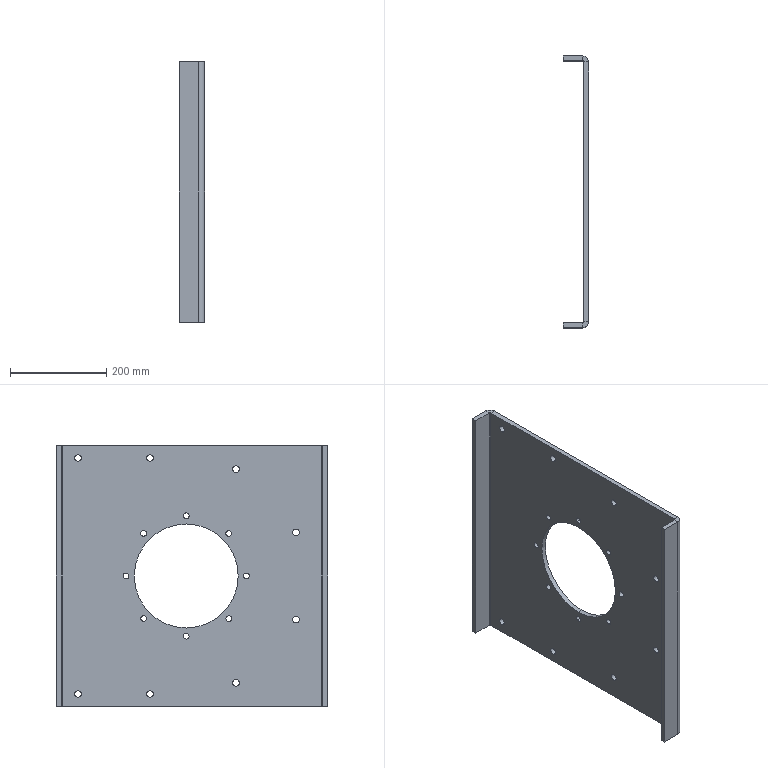Part | STEP file | Input 4 | 1 solid | 56 faces | box 52 x 564 x 540 mm | volume 3076636 mm3 | cylinder 38 | plane 18 | commonest cylinder face diameters 12 x16 14 x16 5 x2 25 x2 216 x2